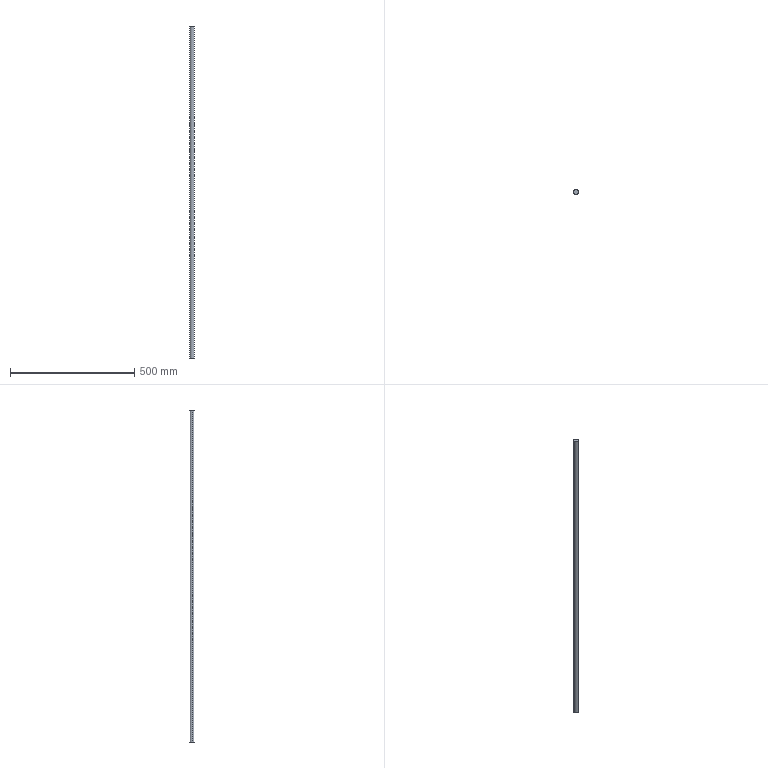Part | STEP file | Part 3^three-axis module | 1 solid | 4 faces | box 20 x 20 x 1337 mm | volume 420031 mm3 | cylinder 2 | plane 2 | commonest cylinder face diameters 20 x2
STEP:
#1=CARTESIAN_POINT('',(-10.,0.,1171.));
#2=VERTEX_POINT('',#1);
#3=CARTESIAN_POINT('',(10.,0.,1171.));
#4=VERTEX_POINT('',#3);
#5=CARTESIAN_POINT('',(0.,0.,1171.));
#6=DIRECTION('',(0.,0.,-1.));
#7=DIRECTION('',(-1.,0.,0.));
#8=AXIS2_PLACEMENT_3D('',#5,#6,#7);
#9=CIRCLE('',#8,10.);
#10=EDGE_CURVE('',#2,#4,#9,.T.);
#11=ORIENTED_EDGE('',*,*,#10,.T.);
#12=CARTESIAN_POINT('',(10.,0.,-166.));
#13=VERTEX_POINT('',#12);
#14=CARTESIAN_POINT('',(10.,0.,1171.));
#15=DIRECTION('',(0.,0.,-1.));
#16=VECTOR('',#15,1000.);
#17=LINE('',#14,#16);
#18=EDGE_CURVE('',#4,#13,#17,.T.);
#19=ORIENTED_EDGE('',*,*,#18,.T.);
#20=CARTESIAN_POINT('',(-10.,0.,-166.));
#21=VERTEX_POINT('',#20);
#22=CARTESIAN_POINT('',(0.,0.,-166.));
#23=DIRECTION('',(0.,0.,1.));
#24=DIRECTION('',(-1.,0.,0.));
#25=AXIS2_PLACEMENT_3D('',#22,#23,#24);
#26=CIRCLE('',#25,10.);
#27=EDGE_CURVE('',#13,#21,#26,.T.);
#28=ORIENTED_EDGE('',*,*,#27,.T.);
#29=CARTESIAN_POINT('',(-10.,0.,1171.));
#30=DIRECTION('',(0.,0.,-1.));
#31=VECTOR('',#30,1000.);
#32=LINE('',#29,#31);
#33=EDGE_CURVE('',#2,#21,#32,.T.);
#34=ORIENTED_EDGE('',*,*,#33,.F.);
#35=EDGE_LOOP('',(#11,#19,#28,#34));
#36=FACE_OUTER_BOUND('',#35,.T.);
#37=CARTESIAN_POINT('',(0.,0.,1171.));
#38=DIRECTION('',(0.,0.,-1.));
#39=DIRECTION('',(-1.,0.,0.));
#40=AXIS2_PLACEMENT_3D('',#37,#38,#39);
#41=CYLINDRICAL_SURFACE('',#40,10.);
#42=ADVANCED_FACE('',(#36),#41,.T.);
#43=ORIENTED_EDGE('',*,*,#18,.F.);
#44=CARTESIAN_POINT('',(0.,0.,1171.));
#45=DIRECTION('',(0.,0.,-1.));
#46=DIRECTION('',(-1.,0.,0.));
#47=AXIS2_PLACEMENT_3D('',#44,#45,#46);
#48=CIRCLE('',#47,10.);
#49=EDGE_CURVE('',#4,#2,#48,.T.);
#50=ORIENTED_EDGE('',*,*,#49,.T.);
#51=ORIENTED_EDGE('',*,*,#33,.T.);
#52=CARTESIAN_POINT('',(0.,0.,-166.));
#53=DIRECTION('',(0.,0.,1.));
#54=DIRECTION('',(-1.,0.,0.));
#55=AXIS2_PLACEMENT_3D('',#52,#53,#54);
#56=CIRCLE('',#55,10.);
#57=EDGE_CURVE('',#21,#13,#56,.T.);
#58=ORIENTED_EDGE('',*,*,#57,.T.);
#59=EDGE_LOOP('',(#43,#50,#51,#58));
#60=FACE_OUTER_BOUND('',#59,.T.);
#61=CARTESIAN_POINT('',(0.,0.,1171.));
#62=DIRECTION('',(0.,0.,-1.));
#63=DIRECTION('',(-1.,0.,0.));
#64=AXIS2_PLACEMENT_3D('',#61,#62,#63);
#65=CYLINDRICAL_SURFACE('',#64,10.);
#66=ADVANCED_FACE('',(#60),#65,.T.);
#67=ORIENTED_EDGE('',*,*,#57,.F.);
#68=ORIENTED_EDGE('',*,*,#27,.F.);
#69=EDGE_LOOP('',(#67,#68));
#70=FACE_OUTER_BOUND('',#69,.T.);
#71=CARTESIAN_POINT('',(0.,0.,-166.));
#72=DIRECTION('',(0.,0.,-1.));
#73=DIRECTION('',(-1.,0.,0.));
#74=AXIS2_PLACEMENT_3D('',#71,#72,#73);
#75=PLANE('',#74);
#76=ADVANCED_FACE('',(#70),#75,.T.);
#77=ORIENTED_EDGE('',*,*,#10,.F.);
#78=ORIENTED_EDGE('',*,*,#49,.F.);
#79=EDGE_LOOP('',(#77,#78));
#80=FACE_OUTER_BOUND('',#79,.T.);
#81=CARTESIAN_POINT('',(0.,0.,1171.));
#82=DIRECTION('',(0.,0.,1.));
#83=DIRECTION('',(1.,0.,0.));
#84=AXIS2_PLACEMENT_3D('',#81,#82,#83);
#85=PLANE('',#84);
#86=ADVANCED_FACE('',(#80),#85,.T.);
#87=CLOSED_SHELL('',(#42,#66,#76,#86));
#88=MANIFOLD_SOLID_BREP('',#87);
#89=CARTESIAN_POINT('',(0.,0.,0.));
#90=DIRECTION('',(0.,0.,1.));
#91=DIRECTION('',(1.,0.,0.));
#92=AXIS2_PLACEMENT_3D('',#89,#90,#91);
#93=(LENGTH_UNIT()NAMED_UNIT(*)SI_UNIT(.MILLI.,.METRE.));
#94=UNCERTAINTY_MEASURE_WITH_UNIT(LENGTH_MEASURE(0.00001),#93,'','');
#95=(NAMED_UNIT(*)PLANE_ANGLE_UNIT()SI_UNIT($,.RADIAN.));
#96=(NAMED_UNIT(*)SI_UNIT($,.STERADIAN.)SOLID_ANGLE_UNIT());
#97=(GEOMETRIC_REPRESENTATION_CONTEXT(3)GLOBAL_UNCERTAINTY_ASSIGNED_CONTEXT((#94))GLOBAL_UNIT_ASSIGNED_CONTEXT((#93,#95,#96))REPRESENTATION_CONTEXT('',''));
#98=ADVANCED_BREP_SHAPE_REPRESENTATION('',(#88,#92),#97);